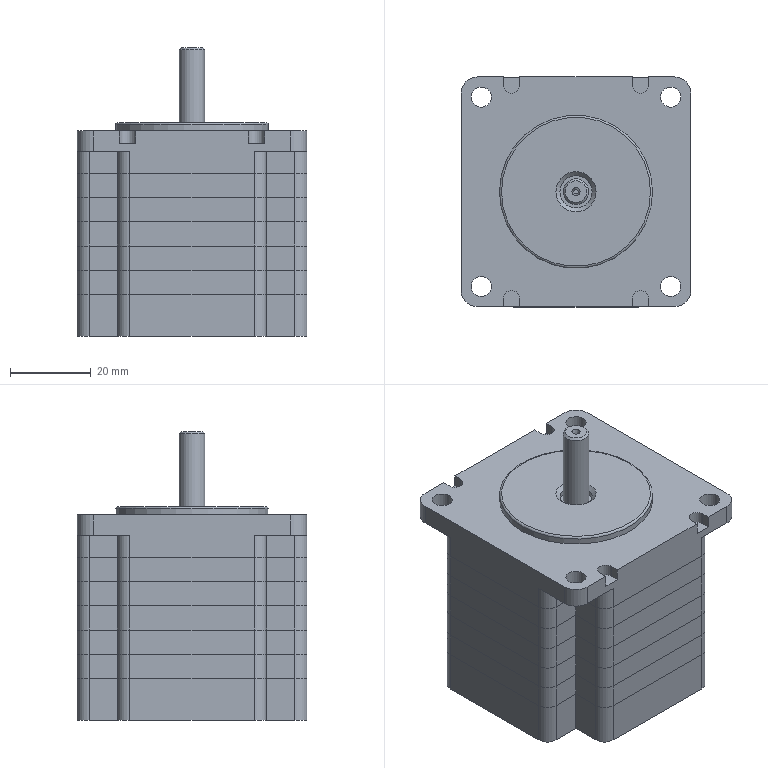Part | STEP file | 57bujindianji | 1 solid | 181 faces | box 57 x 57 x 71.7 mm | volume 148752 mm3 | plane 106 | cylinder 71 | cone 3 | torus 1 | commonest cylinder face diameters 6 x56 8 x5 4 x4 5 x4 6.35 x1 38 x1